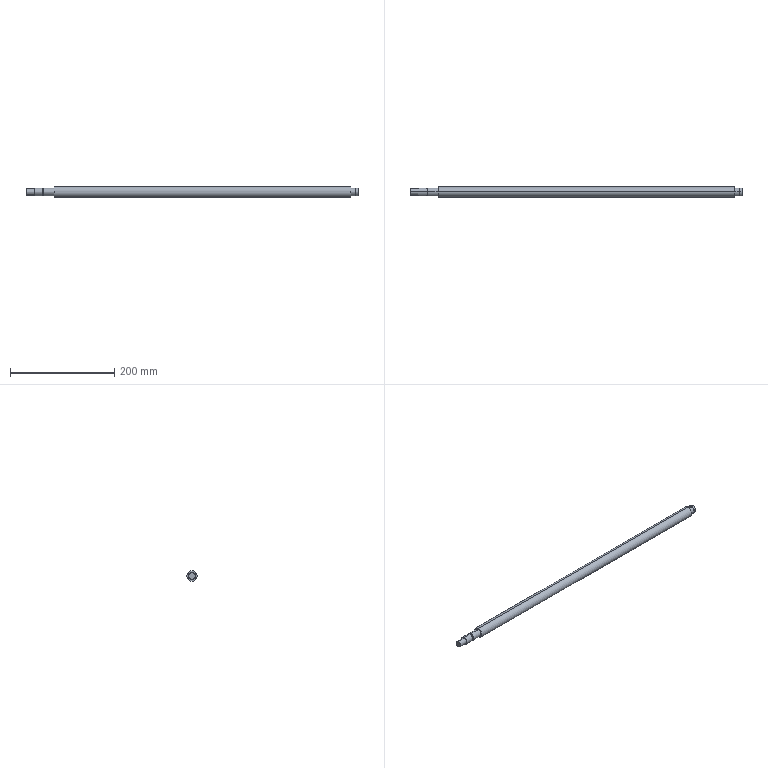Part | STEP file | PN_0055 lead screw 20-5T3 | 1 solid | 25 faces | box 638 x 20 x 20 mm | volume 189984 mm3 | cylinder 16 | plane 9 | commonest cylinder face diameters 15 x8 12 x2 13.5 x2 14.3 x2 20 x2